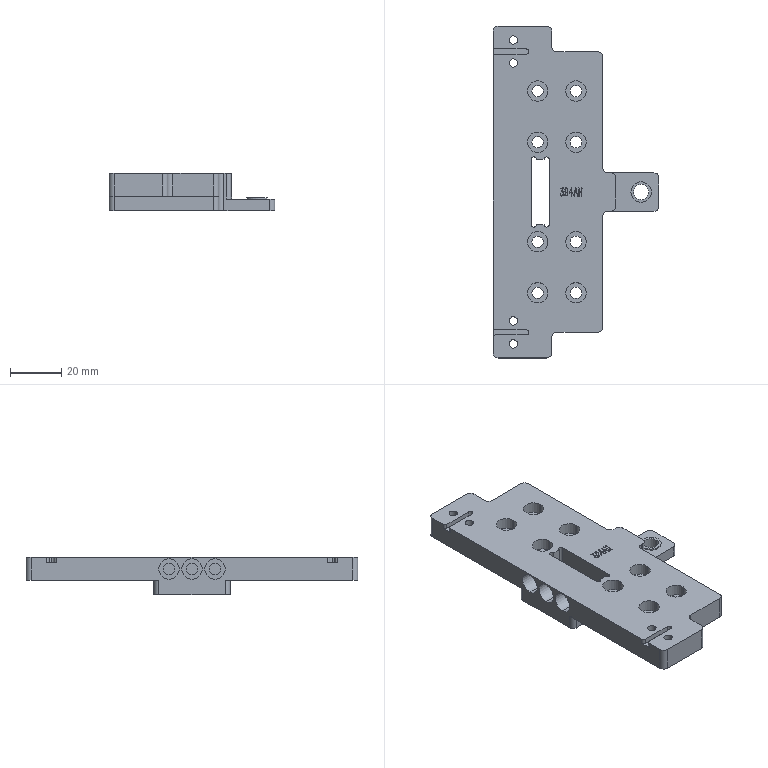NC program | NX | posted with a generic post | part box 65 x 130 x 14.5 mm
Lines 1 to 107 of 11202:
N10 G17 G21 G94 G90
(FLOOR_WALL_COPY , TOOL : D80)
N12 T19 M6
N14 G54
N16 G17 G0 G90 X115. Y0. B0. C0. S6500 M3
N18 G43 Z30. H19
N20 Z3.
N22 G94 G1 Z0. F1500.
N24 X110.
N26 X-110.
N28 X-115.
N30 Z3.
N32 G0 Z30.
N34 M5
(DRILLING_COPY_1 , TOOL : D6A45)
N36 T01 M6
N38 G54
N40 G17 G0 G90 X-59.5 Y-24.5 B0. C0. S5000 M3
N42 G43 Z30. H1
N44 G94 G81 G98 Z-1. F350. R3.
N46 X-50.5
N48 X-39.5 Y-15.
N50 Y0.
N52 X-19.5
N54 Y-15.
N56 X-12.75 Y-16.5
N58 Y-11.5
N60 X12.75
N62 Y-16.5
N64 X19.5 Y-15.
N66 Y0.
N68 X39.5
N70 Y-15.
N72 X50.5 Y-24.5
N74 X59.5
N76 G80
N78 G0 X59.5 Y-24.5 Z30.
(DRILLING_COPY_1_COPY_1 , TOOL : D6A45)
N80 X-59.5
N82 G81 Z-2.1 F350. R3.
N84 X-50.5
N86 X50.5
N88 X59.5
N90 G80
N92 G0 X59.5 Y-24.5 Z30.
N94 M5
(DRILLING_COPY_COPY , TOOL : 3.3ZT)
N96 T03 M6
N98 G54
N100 G17 G0 G90 X-59.5 Y-24.5 B0. C0. S2000 M3
N102 G43 Z30. H3
N104 G94 G83 G98 Z-11.491 F180. Q2. R3.
N106 X-50.5
N108 X50.5
N110 X59.5
N112 G80
N114 G0 X59.5 Y-24.5 Z30.
N116 M5
(DRILLING_COPY_COPY_COPY_2 , TOOL : 4.5ZT)
N118 T08 M6
N120 G54
N122 G17 G0 G90 X-39.5 Y0. B0. C0. S2000 M3
N124 G43 Z30. H8
N126 G94 G83 G98 Z-9.352 F180. Q2. R3.
N128 X-19.5
N130 X19.5
N132 X39.5
N134 X-39.5 Y-15.
N136 X-19.5
N138 X19.5
N140 X39.5
N142 G80
N144 G0 X39.5 Y-15. Z30.
(DRILLING_COPY_COPY_COPY_2_COPY , TOOL : 4.5ZT)
N146 X0. Y25.5
N148 G83 Z-16.852 F180. Q2. R3.
N150 G80
N152 G0 X0. Y25.5 Z30.
N154 M5
(DRILLING_COPY_COPY_COPY_1 , TOOL : 2.0ZT)
N156 T02 M6
N158 G54
N160 G17 G0 G90 X-12.75 Y-11.5 B0. C0. S3000 M3
N162 G43 Z30. H2
N164 G94 G83 G98 Z-16.101 F120. Q2. R3.
N166 Y-16.5
N168 X12.75
N170 Y-11.5
N172 G80
N174 G0 X12.75 Y-11.5 Z30.
N176 M5